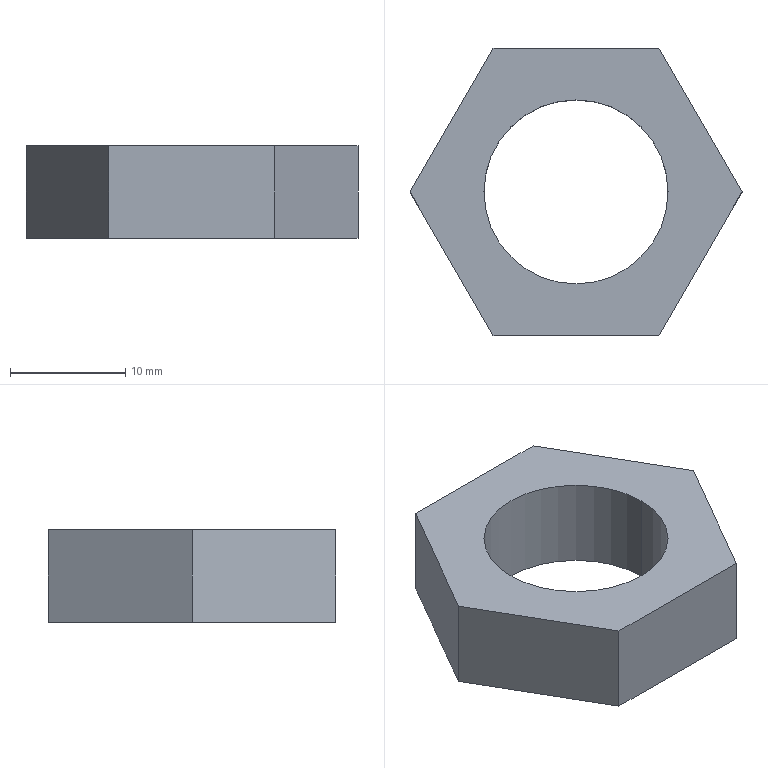Part | STEP file | M16 nut | 1 solid | 10 faces | box 28.868 x 25 x 8 mm | volume 2722 mm3 | plane 8 | cylinder 2 | commonest cylinder face diameters 16 x2
STEP:
#1=CARTESIAN_POINT('',(0.,0.,0.));
#2=DIRECTION('',(0.,0.,1.));
#3=DIRECTION('',(1.,0.,0.));
#4=AXIS2_PLACEMENT_3D('',#1,#2,#3);
#5=CARTESIAN_POINT('',(-8.,0.,8.));
#6=VERTEX_POINT('',#5);
#7=CARTESIAN_POINT('',(-8.,0.,0.));
#8=VERTEX_POINT('',#7);
#9=CARTESIAN_POINT('',(-8.,0.,8.));
#10=DIRECTION('',(0.,0.,-1.));
#11=VECTOR('',#10,1.);
#12=LINE('',#9,#11);
#13=CARTESIAN_POINT('',(0.,0.,8.));
#14=DIRECTION('',(0.,0.,-1.));
#15=DIRECTION('',(-1.,0.,0.));
#16=AXIS2_PLACEMENT_3D('',#13,#14,#15);
#17=CYLINDRICAL_SURFACE('',#16,8.);
#18=CARTESIAN_POINT('',(6.283,0.));
#19=DIRECTION('',(0.,1.));
#20=VECTOR('',#19,1.);
#21=LINE('',#18,#20);
#22=(GEOMETRIC_REPRESENTATION_CONTEXT(2)PARAMETRIC_REPRESENTATION_CONTEXT()REPRESENTATION_CONTEXT('',''));
#23=DEFINITIONAL_REPRESENTATION('',(#21),#22);
#24=PCURVE('',#17,#23);
#25=CARTESIAN_POINT('',(0.,0.,8.));
#26=DIRECTION('',(0.,0.,-1.));
#27=DIRECTION('',(-1.,0.,0.));
#28=AXIS2_PLACEMENT_3D('',#25,#26,#27);
#29=CYLINDRICAL_SURFACE('',#28,8.);
#30=CARTESIAN_POINT('',(0.,0.));
#31=DIRECTION('',(0.,1.));
#32=VECTOR('',#31,1.);
#33=LINE('',#30,#32);
#34=(GEOMETRIC_REPRESENTATION_CONTEXT(2)PARAMETRIC_REPRESENTATION_CONTEXT()REPRESENTATION_CONTEXT('',''));
#35=DEFINITIONAL_REPRESENTATION('',(#33),#34);
#36=PCURVE('',#29,#35);
#37=SURFACE_CURVE('',#12,(#24,#36),.PCURVE_S1.);
#38=EDGE_CURVE('',#6,#8,#37,.T.);
#39=ORIENTED_EDGE('',*,*,#38,.T.);
#40=CARTESIAN_POINT('',(8.,0.,0.));
#41=VERTEX_POINT('',#40);
#42=CARTESIAN_POINT('',(0.,0.,0.));
#43=DIRECTION('',(0.,0.,-1.));
#44=DIRECTION('',(-1.,0.,0.));
#45=AXIS2_PLACEMENT_3D('',#42,#43,#44);
#46=CIRCLE('',#45,8.);
#47=CARTESIAN_POINT('',(0.,8.));
#48=DIRECTION('',(1.,0.));
#49=VECTOR('',#48,1.);
#50=LINE('',#47,#49);
#51=(GEOMETRIC_REPRESENTATION_CONTEXT(2)PARAMETRIC_REPRESENTATION_CONTEXT()REPRESENTATION_CONTEXT('',''));
#52=DEFINITIONAL_REPRESENTATION('',(#50),#51);
#53=PCURVE('',#17,#52);
#54=CARTESIAN_POINT('',(0.,0.,0.));
#55=DIRECTION('',(0.,0.,1.));
#56=DIRECTION('',(1.,0.,0.));
#57=AXIS2_PLACEMENT_3D('',#54,#55,#56);
#58=PLANE('',#57);
#59=CARTESIAN_POINT('',(-8.,0.));
#60=CARTESIAN_POINT('',(-8.,13.856));
#61=CARTESIAN_POINT('',(4.,6.928));
#62=CARTESIAN_POINT('',(16.,0.));
#63=CARTESIAN_POINT('',(4.,-6.928));
#64=CARTESIAN_POINT('',(-8.,-13.856));
#65=CARTESIAN_POINT('',(-8.,0.));
#66=(BOUNDED_CURVE()B_SPLINE_CURVE(2,(#59,#60,#61,#62,#63,#64,#65),.UNSPECIFIED.,.T.,.F.)B_SPLINE_CURVE_WITH_KNOTS((1,2,2,2,2,1),(-2.094,0.,2.094,4.189,6.283,8.378),.UNSPECIFIED.)CURVE()GEOMETRIC_REPRESENTATION_ITEM()RATIONAL_B_SPLINE_CURVE((1.,0.5,1.,0.5,1.,0.5,1.))REPRESENTATION_ITEM(''));
#67=(GEOMETRIC_REPRESENTATION_CONTEXT(2)PARAMETRIC_REPRESENTATION_CONTEXT()REPRESENTATION_CONTEXT('',''));
#68=DEFINITIONAL_REPRESENTATION('',(#66),#67);
#69=PCURVE('',#58,#68);
#70=SURFACE_CURVE('',#46,(#53,#69),.PCURVE_S1.);
#71=EDGE_CURVE('',#41,#8,#70,.T.);
#72=ORIENTED_EDGE('',*,*,#71,.F.);
#73=CARTESIAN_POINT('',(8.,0.,8.));
#74=VERTEX_POINT('',#73);
#75=CARTESIAN_POINT('',(8.,0.,8.));
#76=DIRECTION('',(0.,0.,-1.));
#77=VECTOR('',#76,1.);
#78=LINE('',#75,#77);
#79=CARTESIAN_POINT('',(3.142,0.));
#80=DIRECTION('',(0.,1.));
#81=VECTOR('',#80,1.);
#82=LINE('',#79,#81);
#83=(GEOMETRIC_REPRESENTATION_CONTEXT(2)PARAMETRIC_REPRESENTATION_CONTEXT()REPRESENTATION_CONTEXT('',''));
#84=DEFINITIONAL_REPRESENTATION('',(#82),#83);
#85=PCURVE('',#17,#84);
#86=CARTESIAN_POINT('',(3.142,0.));
#87=DIRECTION('',(0.,1.));
#88=VECTOR('',#87,1.);
#89=LINE('',#86,#88);
#90=(GEOMETRIC_REPRESENTATION_CONTEXT(2)PARAMETRIC_REPRESENTATION_CONTEXT()REPRESENTATION_CONTEXT('',''));
#91=DEFINITIONAL_REPRESENTATION('',(#89),#90);
#92=PCURVE('',#29,#91);
#93=SURFACE_CURVE('',#78,(#85,#92),.PCURVE_S1.);
#94=EDGE_CURVE('',#74,#41,#93,.T.);
#95=ORIENTED_EDGE('',*,*,#94,.F.);
#96=CARTESIAN_POINT('',(0.,0.,8.));
#97=DIRECTION('',(0.,0.,-1.));
#98=DIRECTION('',(-1.,0.,0.));
#99=AXIS2_PLACEMENT_3D('',#96,#97,#98);
#100=CIRCLE('',#99,8.);
#101=CARTESIAN_POINT('',(0.,0.));
#102=DIRECTION('',(1.,0.));
#103=VECTOR('',#102,1.);
#104=LINE('',#101,#103);
#105=(GEOMETRIC_REPRESENTATION_CONTEXT(2)PARAMETRIC_REPRESENTATION_CONTEXT()REPRESENTATION_CONTEXT('',''));
#106=DEFINITIONAL_REPRESENTATION('',(#104),#105);
#107=PCURVE('',#17,#106);
#108=CARTESIAN_POINT('',(0.,0.,8.));
#109=DIRECTION('',(0.,0.,1.));
#110=DIRECTION('',(1.,0.,0.));
#111=AXIS2_PLACEMENT_3D('',#108,#109,#110);
#112=PLANE('',#111);
#113=CARTESIAN_POINT('',(-8.,0.));
#114=CARTESIAN_POINT('',(-8.,13.856));
#115=CARTESIAN_POINT('',(4.,6.928));
#116=CARTESIAN_POINT('',(16.,0.));
#117=CARTESIAN_POINT('',(4.,-6.928));
#118=CARTESIAN_POINT('',(-8.,-13.856));
#119=CARTESIAN_POINT('',(-8.,0.));
#120=(BOUNDED_CURVE()B_SPLINE_CURVE(2,(#113,#114,#115,#116,#117,#118,#119),.UNSPECIFIED.,.T.,.F.)B_SPLINE_CURVE_WITH_KNOTS((1,2,2,2,2,1),(-2.094,0.,2.094,4.189,6.283,8.378),.UNSPECIFIED.)CURVE()GEOMETRIC_REPRESENTATION_ITEM()RATIONAL_B_SPLINE_CURVE((1.,0.5,1.,0.5,1.,0.5,1.))REPRESENTATION_ITEM(''));
#121=(GEOMETRIC_REPRESENTATION_CONTEXT(2)PARAMETRIC_REPRESENTATION_CONTEXT()REPRESENTATION_CONTEXT('',''));
#122=DEFINITIONAL_REPRESENTATION('',(#120),#121);
#123=PCURVE('',#112,#122);
#124=SURFACE_CURVE('',#100,(#107,#123),.PCURVE_S1.);
#125=EDGE_CURVE('',#74,#6,#124,.T.);
#126=ORIENTED_EDGE('',*,*,#125,.T.);
#127=EDGE_LOOP('',(#39,#72,#95,#126));
#128=FACE_BOUND('',#127,.F.);
#129=ADVANCED_FACE('',(#128),#17,.F.);
#130=CARTESIAN_POINT('',(0.,0.,0.));
#131=DIRECTION('',(0.,0.,-1.));
#132=DIRECTION('',(-1.,0.,0.));
#133=AXIS2_PLACEMENT_3D('',#130,#131,#132);
#134=CIRCLE('',#133,8.);
#135=CARTESIAN_POINT('',(-8.,0.));
#136=CARTESIAN_POINT('',(-8.,13.856));
#137=CARTESIAN_POINT('',(4.,6.928));
#138=CARTESIAN_POINT('',(16.,0.));
#139=CARTESIAN_POINT('',(4.,-6.928));
#140=CARTESIAN_POINT('',(-8.,-13.856));
#141=CARTESIAN_POINT('',(-8.,0.));
#142=(BOUNDED_CURVE()B_SPLINE_CURVE(2,(#135,#136,#137,#138,#139,#140,#141),.UNSPECIFIED.,.T.,.F.)B_SPLINE_CURVE_WITH_KNOTS((1,2,2,2,2,1),(-2.094,0.,2.094,4.189,6.283,8.378),.UNSPECIFIED.)CURVE()GEOMETRIC_REPRESENTATION_ITEM()RATIONAL_B_SPLINE_CURVE((1.,0.5,1.,0.5,1.,0.5,1.))REPRESENTATION_ITEM(''));
#143=(GEOMETRIC_REPRESENTATION_CONTEXT(2)PARAMETRIC_REPRESENTATION_CONTEXT()REPRESENTATION_CONTEXT('',''));
#144=DEFINITIONAL_REPRESENTATION('',(#142),#143);
#145=PCURVE('',#58,#144);
#146=CARTESIAN_POINT('',(0.,8.));
#147=DIRECTION('',(1.,0.));
#148=VECTOR('',#147,1.);
#149=LINE('',#146,#148);
#150=(GEOMETRIC_REPRESENTATION_CONTEXT(2)PARAMETRIC_REPRESENTATION_CONTEXT()REPRESENTATION_CONTEXT('',''));
#151=DEFINITIONAL_REPRESENTATION('',(#149),#150);
#152=PCURVE('',#29,#151);
#153=SURFACE_CURVE('',#134,(#145,#152),.PCURVE_S1.);
#154=EDGE_CURVE('',#8,#41,#153,.T.);
#155=ORIENTED_EDGE('',*,*,#154,.F.);
#156=ORIENTED_EDGE('',*,*,#71,.F.);
#157=EDGE_LOOP('',(#155,#156));
#158=FACE_BOUND('',#157,.T.);
#159=CARTESIAN_POINT('',(-7.217,-12.5,0.));
#160=VERTEX_POINT('',#159);
#161=CARTESIAN_POINT('',(7.217,-12.5,0.));
#162=VERTEX_POINT('',#161);
#163=CARTESIAN_POINT('',(0.,-12.5,0.));
#164=DIRECTION('',(1.,0.,0.));
#165=VECTOR('',#164,1.);
#166=LINE('',#163,#165);
#167=CARTESIAN_POINT('',(0.,-12.5));
#168=DIRECTION('',(1.,0.));
#169=VECTOR('',#168,1.);
#170=LINE('',#167,#169);
#171=(GEOMETRIC_REPRESENTATION_CONTEXT(2)PARAMETRIC_REPRESENTATION_CONTEXT()REPRESENTATION_CONTEXT('',''));
#172=DEFINITIONAL_REPRESENTATION('',(#170),#171);
#173=PCURVE('',#58,#172);
#174=CARTESIAN_POINT('',(-7.217,-12.5,8.));
#175=DIRECTION('',(0.,1.,0.));
#176=DIRECTION('',(0.,0.,1.));
#177=AXIS2_PLACEMENT_3D('',#174,#175,#176);
#178=PLANE('',#177);
#179=CARTESIAN_POINT('',(-8.,7.217));
#180=DIRECTION('',(0.,1.));
#181=VECTOR('',#180,1.);
#182=LINE('',#179,#181);
#183=(GEOMETRIC_REPRESENTATION_CONTEXT(2)PARAMETRIC_REPRESENTATION_CONTEXT()REPRESENTATION_CONTEXT('',''));
#184=DEFINITIONAL_REPRESENTATION('',(#182),#183);
#185=PCURVE('',#178,#184);
#186=SURFACE_CURVE('',#166,(#173,#185),.PCURVE_S1.);
#187=EDGE_CURVE('',#160,#162,#186,.T.);
#188=ORIENTED_EDGE('',*,*,#187,.F.);
#189=CARTESIAN_POINT('',(-14.434,0.,0.));
#190=VERTEX_POINT('',#189);
#191=CARTESIAN_POINT('',(-14.434,0.,0.));
#192=DIRECTION('',(0.5,-0.866,0.));
#193=VECTOR('',#192,1.);
#194=LINE('',#191,#193);
#195=CARTESIAN_POINT('',(-14.434,0.));
#196=DIRECTION('',(0.5,-0.866));
#197=VECTOR('',#196,1.);
#198=LINE('',#195,#197);
#199=(GEOMETRIC_REPRESENTATION_CONTEXT(2)PARAMETRIC_REPRESENTATION_CONTEXT()REPRESENTATION_CONTEXT('',''));
#200=DEFINITIONAL_REPRESENTATION('',(#198),#199);
#201=PCURVE('',#58,#200);
#202=CARTESIAN_POINT('',(-14.434,0.,8.));
#203=DIRECTION('',(0.866,0.5,0.));
#204=DIRECTION('',(-0.5,0.866,0.));
#205=AXIS2_PLACEMENT_3D('',#202,#203,#204);
#206=PLANE('',#205);
#207=CARTESIAN_POINT('',(0.,-8.));
#208=DIRECTION('',(-1.,0.));
#209=VECTOR('',#208,1.);
#210=LINE('',#207,#209);
#211=(GEOMETRIC_REPRESENTATION_CONTEXT(2)PARAMETRIC_REPRESENTATION_CONTEXT()REPRESENTATION_CONTEXT('',''));
#212=DEFINITIONAL_REPRESENTATION('',(#210),#211);
#213=PCURVE('',#206,#212);
#214=SURFACE_CURVE('',#194,(#201,#213),.PCURVE_S1.);
#215=EDGE_CURVE('',#190,#160,#214,.T.);
#216=ORIENTED_EDGE('',*,*,#215,.F.);
#217=CARTESIAN_POINT('',(-7.217,12.5,0.));
#218=VERTEX_POINT('',#217);
#219=CARTESIAN_POINT('',(-7.217,12.5,0.));
#220=DIRECTION('',(-0.5,-0.866,0.));
#221=VECTOR('',#220,1.);
#222=LINE('',#219,#221);
#223=CARTESIAN_POINT('',(-7.217,12.5));
#224=DIRECTION('',(-0.5,-0.866));
#225=VECTOR('',#224,1.);
#226=LINE('',#223,#225);
#227=(GEOMETRIC_REPRESENTATION_CONTEXT(2)PARAMETRIC_REPRESENTATION_CONTEXT()REPRESENTATION_CONTEXT('',''));
#228=DEFINITIONAL_REPRESENTATION('',(#226),#227);
#229=PCURVE('',#58,#228);
#230=CARTESIAN_POINT('',(-7.217,12.5,8.));
#231=DIRECTION('',(0.866,-0.5,0.));
#232=DIRECTION('',(0.5,0.866,0.));
#233=AXIS2_PLACEMENT_3D('',#230,#231,#232);
#234=PLANE('',#233);
#235=CARTESIAN_POINT('',(0.,-8.));
#236=DIRECTION('',(-1.,0.));
#237=VECTOR('',#236,1.);
#238=LINE('',#235,#237);
#239=(GEOMETRIC_REPRESENTATION_CONTEXT(2)PARAMETRIC_REPRESENTATION_CONTEXT()REPRESENTATION_CONTEXT('',''));
#240=DEFINITIONAL_REPRESENTATION('',(#238),#239);
#241=PCURVE('',#234,#240);
#242=SURFACE_CURVE('',#222,(#229,#241),.PCURVE_S1.);
#243=EDGE_CURVE('',#218,#190,#242,.T.);
#244=ORIENTED_EDGE('',*,*,#243,.F.);
#245=CARTESIAN_POINT('',(7.217,12.5,0.));
#246=VERTEX_POINT('',#245);
#247=CARTESIAN_POINT('',(0.,12.5,0.));
#248=DIRECTION('',(-1.,0.,0.));
#249=VECTOR('',#248,1.);
#250=LINE('',#247,#249);
#251=CARTESIAN_POINT('',(0.,12.5));
#252=DIRECTION('',(-1.,0.));
#253=VECTOR('',#252,1.);
#254=LINE('',#251,#253);
#255=(GEOMETRIC_REPRESENTATION_CONTEXT(2)PARAMETRIC_REPRESENTATION_CONTEXT()REPRESENTATION_CONTEXT('',''));
#256=DEFINITIONAL_REPRESENTATION('',(#254),#255);
#257=PCURVE('',#58,#256);
#258=CARTESIAN_POINT('',(7.217,12.5,8.));
#259=DIRECTION('',(0.,-1.,0.));
#260=DIRECTION('',(0.,0.,-1.));
#261=AXIS2_PLACEMENT_3D('',#258,#259,#260);
#262=PLANE('',#261);
#263=CARTESIAN_POINT('',(8.,-7.217));
#264=DIRECTION('',(0.,-1.));
#265=VECTOR('',#264,1.);
#266=LINE('',#263,#265);
#267=(GEOMETRIC_REPRESENTATION_CONTEXT(2)PARAMETRIC_REPRESENTATION_CONTEXT()REPRESENTATION_CONTEXT('',''));
#268=DEFINITIONAL_REPRESENTATION('',(#266),#267);
#269=PCURVE('',#262,#268);
#270=SURFACE_CURVE('',#250,(#257,#269),.PCURVE_S1.);
#271=EDGE_CURVE('',#246,#218,#270,.T.);
#272=ORIENTED_EDGE('',*,*,#271,.F.);
#273=CARTESIAN_POINT('',(14.434,0.,0.));
#274=VERTEX_POINT('',#273);
#275=CARTESIAN_POINT('',(14.434,0.,0.));
#276=DIRECTION('',(-0.5,0.866,0.));
#277=VECTOR('',#276,1.);
#278=LINE('',#275,#277);
#279=CARTESIAN_POINT('',(14.434,0.));
#280=DIRECTION('',(-0.5,0.866));
#281=VECTOR('',#280,1.);
#282=LINE('',#279,#281);
#283=(GEOMETRIC_REPRESENTATION_CONTEXT(2)PARAMETRIC_REPRESENTATION_CONTEXT()REPRESENTATION_CONTEXT('',''));
#284=DEFINITIONAL_REPRESENTATION('',(#282),#283);
#285=PCURVE('',#58,#284);
#286=CARTESIAN_POINT('',(14.434,0.,8.));
#287=DIRECTION('',(-0.866,-0.5,0.));
#288=DIRECTION('',(0.5,-0.866,0.));
#289=AXIS2_PLACEMENT_3D('',#286,#287,#288);
#290=PLANE('',#289);
#291=CARTESIAN_POINT('',(0.,-8.));
#292=DIRECTION('',(-1.,0.));
#293=VECTOR('',#292,1.);
#294=LINE('',#291,#293);
#295=(GEOMETRIC_REPRESENTATION_CONTEXT(2)PARAMETRIC_REPRESENTATION_CONTEXT()REPRESENTATION_CONTEXT('',''));
#296=DEFINITIONAL_REPRESENTATION('',(#294),#295);
#297=PCURVE('',#290,#296);
#298=SURFACE_CURVE('',#278,(#285,#297),.PCURVE_S1.);
#299=EDGE_CURVE('',#274,#246,#298,.T.);
#300=ORIENTED_EDGE('',*,*,#299,.F.);
#301=CARTESIAN_POINT('',(7.217,-12.5,0.));
#302=DIRECTION('',(0.5,0.866,0.));
#303=VECTOR('',#302,1.);
#304=LINE('',#301,#303);
#305=CARTESIAN_POINT('',(7.217,-12.5));
#306=DIRECTION('',(0.5,0.866));
#307=VECTOR('',#306,1.);
#308=LINE('',#305,#307);
#309=(GEOMETRIC_REPRESENTATION_CONTEXT(2)PARAMETRIC_REPRESENTATION_CONTEXT()REPRESENTATION_CONTEXT('',''));
#310=DEFINITIONAL_REPRESENTATION('',(#308),#309);
#311=PCURVE('',#58,#310);
#312=CARTESIAN_POINT('',(7.217,-12.5,8.));
#313=DIRECTION('',(-0.866,0.5,0.));
#314=DIRECTION('',(-0.5,-0.866,0.));
#315=AXIS2_PLACEMENT_3D('',#312,#313,#314);
#316=PLANE('',#315);
#317=CARTESIAN_POINT('',(0.,-8.));
#318=DIRECTION('',(-1.,0.));
#319=VECTOR('',#318,1.);
#320=LINE('',#317,#319);
#321=(GEOMETRIC_REPRESENTATION_CONTEXT(2)PARAMETRIC_REPRESENTATION_CONTEXT()REPRESENTATION_CONTEXT('',''));
#322=DEFINITIONAL_REPRESENTATION('',(#320),#321);
#323=PCURVE('',#316,#322);
#324=SURFACE_CURVE('',#304,(#311,#323),.PCURVE_S1.);
#325=EDGE_CURVE('',#162,#274,#324,.T.);
#326=ORIENTED_EDGE('',*,*,#325,.F.);
#327=EDGE_LOOP('',(#188,#216,#244,#272,#300,#326));
#328=FACE_BOUND('',#327,.T.);
#329=ADVANCED_FACE('',(#158,#328),#58,.F.);
#330=ORIENTED_EDGE('',*,*,#154,.F.);
#331=ORIENTED_EDGE('',*,*,#38,.F.);
#332=CARTESIAN_POINT('',(0.,0.,8.));
#333=DIRECTION('',(0.,0.,-1.));
#334=DIRECTION('',(-1.,0.,0.));
#335=AXIS2_PLACEMENT_3D('',#332,#333,#334);
#336=CIRCLE('',#335,8.);
#337=CARTESIAN_POINT('',(0.,0.));
#338=DIRECTION('',(1.,0.));
#339=VECTOR('',#338,1.);
#340=LINE('',#337,#339);
#341=(GEOMETRIC_REPRESENTATION_CONTEXT(2)PARAMETRIC_REPRESENTATION_CONTEXT()REPRESENTATION_CONTEXT('',''));
#342=DEFINITIONAL_REPRESENTATION('',(#340),#341);
#343=PCURVE('',#29,#342);
#344=CARTESIAN_POINT('',(-8.,0.));
#345=CARTESIAN_POINT('',(-8.,13.856));
#346=CARTESIAN_POINT('',(4.,6.928));
#347=CARTESIAN_POINT('',(16.,0.));
#348=CARTESIAN_POINT('',(4.,-6.928));
#349=CARTESIAN_POINT('',(-8.,-13.856));
#350=CARTESIAN_POINT('',(-8.,0.));
#351=(BOUNDED_CURVE()B_SPLINE_CURVE(2,(#344,#345,#346,#347,#348,#349,#350),.UNSPECIFIED.,.T.,.F.)B_SPLINE_CURVE_WITH_KNOTS((1,2,2,2,2,1),(-2.094,0.,2.094,4.189,6.283,8.378),.UNSPECIFIED.)CURVE()GEOMETRIC_REPRESENTATION_ITEM()RATIONAL_B_SPLINE_CURVE((1.,0.5,1.,0.5,1.,0.5,1.))REPRESENTATION_ITEM(''));
#352=(GEOMETRIC_REPRESENTATION_CONTEXT(2)PARAMETRIC_REPRESENTATION_CONTEXT()REPRESENTATION_CONTEXT('',''));
#353=DEFINITIONAL_REPRESENTATION('',(#351),#352);
#354=PCURVE('',#112,#353);
#355=SURFACE_CURVE('',#336,(#343,#354),.PCURVE_S1.);
#356=EDGE_CURVE('',#6,#74,#355,.T.);
#357=ORIENTED_EDGE('',*,*,#356,.T.);
#358=ORIENTED_EDGE('',*,*,#94,.T.);
#359=EDGE_LOOP('',(#330,#331,#357,#358));
#360=FACE_BOUND('',#359,.F.);
#361=ADVANCED_FACE('',(#360),#29,.F.);
#362=CARTESIAN_POINT('',(14.434,0.,8.));
#363=VERTEX_POINT('',#362);
#364=CARTESIAN_POINT('',(14.434,0.,8.));
#365=DIRECTION('',(0.,0.,-1.));
#366=VECTOR('',#365,1.);
#367=LINE('',#364,#366);
#368=CARTESIAN_POINT('',(-14.434,0.));
#369=DIRECTION('',(0.,-1.));
#370=VECTOR('',#369,1.);
#371=LINE('',#368,#370);
#372=(GEOMETRIC_REPRESENTATION_CONTEXT(2)PARAMETRIC_REPRESENTATION_CONTEXT()REPRESENTATION_CONTEXT('',''));
#373=DEFINITIONAL_REPRESENTATION('',(#371),#372);
#374=PCURVE('',#316,#373);
#375=CARTESIAN_POINT('',(0.,0.));
#376=DIRECTION('',(0.,-1.));
#377=VECTOR('',#376,1.);
#378=LINE('',#375,#377);
#379=(GEOMETRIC_REPRESENTATION_CONTEXT(2)PARAMETRIC_REPRESENTATION_CONTEXT()REPRESENTATION_CONTEXT('',''));
#380=DEFINITIONAL_REPRESENTATION('',(#378),#379);
#381=PCURVE('',#290,#380);
#382=SURFACE_CURVE('',#367,(#374,#381),.PCURVE_S1.);
#383=EDGE_CURVE('',#363,#274,#382,.T.);
#384=ORIENTED_EDGE('',*,*,#383,.F.);
#385=CARTESIAN_POINT('',(7.217,-12.5,8.));
#386=VERTEX_POINT('',#385);
#387=CARTESIAN_POINT('',(7.217,-12.5,8.));
#388=DIRECTION('',(0.5,0.866,0.));
#389=VECTOR('',#388,1.);
#390=LINE('',#387,#389);
#391=CARTESIAN_POINT('',(0.,0.));
#392=DIRECTION('',(-1.,0.));
#393=VECTOR('',#392,1.);
#394=LINE('',#391,#393);
#395=(GEOMETRIC_REPRESENTATION_CONTEXT(2)PARAMETRIC_REPRESENTATION_CONTEXT()REPRESENTATION_CONTEXT('',''));
#396=DEFINITIONAL_REPRESENTATION('',(#394),#395);
#397=PCURVE('',#316,#396);
#398=CARTESIAN_POINT('',(7.217,-12.5));
#399=DIRECTION('',(0.5,0.866));
#400=VECTOR('',#399,1.);
#401=LINE('',#398,#400);
#402=(GEOMETRIC_REPRESENTATION_CONTEXT(2)PARAMETRIC_REPRESENTATION_CONTEXT()REPRESENTATION_CONTEXT('',''));
#403=DEFINITIONAL_REPRESENTATION('',(#401),#402);
#404=PCURVE('',#112,#403);
#405=SURFACE_CURVE('',#390,(#397,#404),.PCURVE_S1.);
#406=EDGE_CURVE('',#386,#363,#405,.T.);
#407=ORIENTED_EDGE('',*,*,#406,.F.);
#408=CARTESIAN_POINT('',(7.217,-12.5,8.));
#409=DIRECTION('',(0.,0.,1.));
#410=VECTOR('',#409,1.);
#411=LINE('',#408,#410);
#412=CARTESIAN_POINT('',(0.,0.));
#413=DIRECTION('',(0.,1.));
#414=VECTOR('',#413,1.);
#415=LINE('',#412,#414);
#416=(GEOMETRIC_REPRESENTATION_CONTEXT(2)PARAMETRIC_REPRESENTATION_CONTEXT()REPRESENTATION_CONTEXT('',''));
#417=DEFINITIONAL_REPRESENTATION('',(#415),#416);
#418=PCURVE('',#316,#417);
#419=CARTESIAN_POINT('',(0.,14.434));
#420=DIRECTION('',(1.,0.));
#421=VECTOR('',#420,1.);
#422=LINE('',#419,#421);
#423=(GEOMETRIC_REPRESENTATION_CONTEXT(2)PARAMETRIC_REPRESENTATION_CONTEXT()REPRESENTATION_CONTEXT('',''));
#424=DEFINITIONAL_REPRESENTATION('',(#422),#423);
#425=PCURVE('',#178,#424);
#426=SURFACE_CURVE('',#411,(#418,#425),.PCURVE_S1.);
#427=EDGE_CURVE('',#162,#386,#426,.T.);
#428=ORIENTED_EDGE('',*,*,#427,.F.);
#429=ORIENTED_EDGE('',*,*,#325,.T.);
#430=EDGE_LOOP('',(#384,#407,#428,#429));
#431=FACE_BOUND('',#430,.T.);
#432=ADVANCED_FACE('',(#431),#316,.F.);
#433=ORIENTED_EDGE('',*,*,#427,.T.);
#434=CARTESIAN_POINT('',(-7.217,-12.5,8.));
#435=VERTEX_POINT('',#434);
#436=CARTESIAN_POINT('',(-7.217,-12.5,8.));
#437=DIRECTION('',(1.,0.,0.));
#438=VECTOR('',#437,1.);
#439=LINE('',#436,#438);
#440=CARTESIAN_POINT('',(0.,0.));
#441=DIRECTION('',(0.,1.));
#442=VECTOR('',#441,1.);
#443=LINE('',#440,#442);
#444=(GEOMETRIC_REPRESENTATION_CONTEXT(2)PARAMETRIC_REPRESENTATION_CONTEXT()REPRESENTATION_CONTEXT('',''));
#445=DEFINITIONAL_REPRESENTATION('',(#443),#444);
#446=PCURVE('',#178,#445);
#447=CARTESIAN_POINT('',(-7.217,-12.5));
#448=DIRECTION('',(1.,0.));
#449=VECTOR('',#448,1.);
#450=LINE('',#447,#449);
#451=(GEOMETRIC_REPRESENTATION_CONTEXT(2)PARAMETRIC_REPRESENTATION_CONTEXT()REPRESENTATION_CONTEXT('',''));
#452=DEFINITIONAL_REPRESENTATION('',(#450),#451);
#453=PCURVE('',#112,#452);
#454=SURFACE_CURVE('',#439,(#446,#453),.PCURVE_S1.);
#455=EDGE_CURVE('',#435,#386,#454,.T.);
#456=ORIENTED_EDGE('',*,*,#455,.F.);
#457=CARTESIAN_POINT('',(-7.217,-12.5,8.));
#458=DIRECTION('',(0.,0.,1.));
#459=VECTOR('',#458,1.);
#460=LINE('',#457,#459);
#461=CARTESIAN_POINT('',(0.,0.));
#462=DIRECTION('',(1.,0.));
#463=VECTOR('',#462,1.);
#464=LINE('',#461,#463);
#465=(GEOMETRIC_REPRESENTATION_CONTEXT(2)PARAMETRIC_REPRESENTATION_CONTEXT()REPRESENTATION_CONTEXT('',''));
#466=DEFINITIONAL_REPRESENTATION('',(#464),#465);
#467=PCURVE('',#178,#466);
#468=CARTESIAN_POINT('',(-14.434,0.));
#469=DIRECTION('',(0.,1.));
#470=VECTOR('',#469,1.);
#471=LINE('',#468,#470);
#472=(GEOMETRIC_REPRESENTATION_CONTEXT(2)PARAMETRIC_REPRESENTATION_CONTEXT()REPRESENTATION_CONTEXT('',''));
#473=DEFINITIONAL_REPRESENTATION('',(#471),#472);
#474=PCURVE('',#206,#473);
#475=SURFACE_CURVE('',#460,(#467,#474),.PCURVE_S1.);
#476=EDGE_CURVE('',#160,#435,#475,.T.);
#477=ORIENTED_EDGE('',*,*,#476,.F.);
#478=ORIENTED_EDGE('',*,*,#187,.T.);
#479=EDGE_LOOP('',(#433,#456,#477,#478));
#480=FACE_BOUND('',#479,.T.);
#481=ADVANCED_FACE('',(#480),#178,.F.);
#482=ORIENTED_EDGE('',*,*,#476,.T.);
#483=CARTESIAN_POINT('',(-14.434,0.,8.));
#484=VERTEX_POINT('',#483);
#485=CARTESIAN_POINT('',(-14.434,0.,8.));
#486=DIRECTION('',(0.5,-0.866,0.));
#487=VECTOR('',#486,1.);
#488=LINE('',#485,#487);
#489=CARTESIAN_POINT('',(0.,0.));
#490=DIRECTION('',(-1.,0.));
#491=VECTOR('',#490,1.);
#492=LINE('',#489,#491);
#493=(GEOMETRIC_REPRESENTATION_CONTEXT(2)PARAMETRIC_REPRESENTATION_CONTEXT()REPRESENTATION_CONTEXT('',''));
#494=DEFINITIONAL_REPRESENTATION('',(#492),#493);
#495=PCURVE('',#206,#494);
#496=CARTESIAN_POINT('',(-14.434,0.));
#497=DIRECTION('',(0.5,-0.866));
#498=VECTOR('',#497,1.);
#499=LINE('',#496,#498);
#500=(GEOMETRIC_REPRESENTATION_CONTEXT(2)PARAMETRIC_REPRESENTATION_CONTEXT()REPRESENTATION_CONTEXT('',''));
#501=DEFINITIONAL_REPRESENTATION('',(#499),#500);
#502=PCURVE('',#112,#501);
#503=SURFACE_CURVE('',#488,(#495,#502),.PCURVE_S1.);
#504=EDGE_CURVE('',#484,#435,#503,.T.);
#505=ORIENTED_EDGE('',*,*,#504,.F.);
#506=CARTESIAN_POINT('',(-14.434,0.,8.));
#507=DIRECTION('',(0.,0.,1.));
#508=VECTOR('',#507,1.);
#509=LINE('',#506,#508);
#510=CARTESIAN_POINT('',(0.,0.));
#511=DIRECTION('',(0.,1.));
#512=VECTOR('',#511,1.);
#513=LINE('',#510,#512);
#514=(GEOMETRIC_REPRESENTATION_CONTEXT(2)PARAMETRIC_REPRESENTATION_CONTEXT()REPRESENTATION_CONTEXT('',''));
#515=DEFINITIONAL_REPRESENTATION('',(#513),#514);
#516=PCURVE('',#206,#515);
#517=CARTESIAN_POINT('',(-14.434,0.));
#518=DIRECTION('',(0.,1.));
#519=VECTOR('',#518,1.);
#520=LINE('',#517,#519);
#521=(GEOMETRIC_REPRESENTATION_CONTEXT(2)PARAMETRIC_REPRESENTATION_CONTEXT()REPRESENTATION_CONTEXT('',''));
#522=DEFINITIONAL_REPRESENTATION('',(#520),#521);
#523=PCURVE('',#234,#522);
#524=SURFACE_CURVE('',#509,(#516,#523),.PCURVE_S1.);
#525=EDGE_CURVE('',#190,#484,#524,.T.);
#526=ORIENTED_EDGE('',*,*,#525,.F.);
#527=ORIENTED_EDGE('',*,*,#215,.T.);
#528=EDGE_LOOP('',(#482,#505,#526,#527));
#529=FACE_BOUND('',#528,.T.);
#530=ADVANCED_FACE('',(#529),#206,.F.);
#531=ORIENTED_EDGE('',*,*,#525,.T.);
#532=CARTESIAN_POINT('',(-7.217,12.5,8.));
#533=VERTEX_POINT('',#532);
#534=CARTESIAN_POINT('',(-7.217,12.5,8.));
#535=DIRECTION('',(-0.5,-0.866,0.));
#536=VECTOR('',#535,1.);
#537=LINE('',#534,#536);
#538=CARTESIAN_POINT('',(0.,0.));
#539=DIRECTION('',(-1.,0.));
#540=VECTOR('',#539,1.);
#541=LINE('',#538,#540);
#542=(GEOMETRIC_REPRESENTATION_CONTEXT(2)PARAMETRIC_REPRESENTATION_CONTEXT()REPRESENTATION_CONTEXT('',''));
#543=DEFINITIONAL_REPRESENTATION('',(#541),#542);
#544=PCURVE('',#234,#543);
#545=CARTESIAN_POINT('',(-7.217,12.5));
#546=DIRECTION('',(-0.5,-0.866));
#547=VECTOR('',#546,1.);
#548=LINE('',#545,#547);
#549=(GEOMETRIC_REPRESENTATION_CONTEXT(2)PARAMETRIC_REPRESENTATION_CONTEXT()REPRESENTATION_CONTEXT('',''));
#550=DEFINITIONAL_REPRESENTATION('',(#548),#549);
#551=PCURVE('',#112,#550);
#552=SURFACE_CURVE('',#537,(#544,#551),.PCURVE_S1.);
#553=EDGE_CURVE('',#533,#484,#552,.T.);
#554=ORIENTED_EDGE('',*,*,#553,.F.);
#555=CARTESIAN_POINT('',(-7.217,12.5,8.));
#556=DIRECTION('',(0.,0.,1.));
#557=VECTOR('',#556,1.);
#558=LINE('',#555,#557);
#559=CARTESIAN_POINT('',(0.,0.));
#560=DIRECTION('',(0.,1.));
#561=VECTOR('',#560,1.);
#562=LINE('',#559,#561);
#563=(GEOMETRIC_REPRESENTATION_CONTEXT(2)PARAMETRIC_REPRESENTATION_CONTEXT()REPRESENTATION_CONTEXT('',''));
#564=DEFINITIONAL_REPRESENTATION('',(#562),#563);
#565=PCURVE('',#234,#564);
#566=CARTESIAN_POINT('',(0.,-14.434));
#567=DIRECTION('',(-1.,0.));
#568=VECTOR('',#567,1.);
#569=LINE('',#566,#568);
#570=(GEOMETRIC_REPRESENTATION_CONTEXT(2)PARAMETRIC_REPRESENTATION_CONTEXT()REPRESENTATION_CONTEXT('',''));
#571=DEFINITIONAL_REPRESENTATION('',(#569),#570);
#572=PCURVE('',#262,#571);
#573=SURFACE_CURVE('',#558,(#565,#572),.PCURVE_S1.);
#574=EDGE_CURVE('',#218,#533,#573,.T.);
#575=ORIENTED_EDGE('',*,*,#574,.F.);
#576=ORIENTED_EDGE('',*,*,#243,.T.);
#577=EDGE_LOOP('',(#531,#554,#575,#576));
#578=FACE_BOUND('',#577,.T.);
#579=ADVANCED_FACE('',(#578),#234,.F.);
#580=ORIENTED_EDGE('',*,*,#574,.T.);
#581=CARTESIAN_POINT('',(7.217,12.5,8.));
#582=VERTEX_POINT('',#581);
#583=CARTESIAN_POINT('',(7.217,12.5,8.));
#584=DIRECTION('',(-1.,0.,0.));
#585=VECTOR('',#584,1.);
#586=LINE('',#583,#585);
#587=CARTESIAN_POINT('',(0.,0.));
#588=DIRECTION('',(0.,-1.));
#589=VECTOR('',#588,1.);
#590=LINE('',#587,#589);
#591=(GEOMETRIC_REPRESENTATION_CONTEXT(2)PARAMETRIC_REPRESENTATION_CONTEXT()REPRESENTATION_CONTEXT('',''));
#592=DEFINITIONAL_REPRESENTATION('',(#590),#591);
#593=PCURVE('',#262,#592);
#594=CARTESIAN_POINT('',(7.217,12.5));
#595=DIRECTION('',(-1.,0.));
#596=VECTOR('',#595,1.);
#597=LINE('',#594,#596);
#598=(GEOMETRIC_REPRESENTATION_CONTEXT(2)PARAMETRIC_REPRESENTATION_CONTEXT()REPRESENTATION_CONTEXT('',''));
#599=DEFINITIONAL_REPRESENTATION('',(#597),#598);
#600=PCURVE('',#112,#599);
#601=SURFACE_CURVE('',#586,(#593,#600),.PCURVE_S1.);
#602=EDGE_CURVE('',#582,#533,#601,.T.);
#603=ORIENTED_EDGE('',*,*,#602,.F.);
#604=CARTESIAN_POINT('',(7.217,12.5,8.));
#605=DIRECTION('',(0.,0.,1.));
#606=VECTOR('',#605,1.);
#607=LINE('',#604,#606);
#608=CARTESIAN_POINT('',(0.,0.));
#609=DIRECTION('',(-1.,0.));
#610=VECTOR('',#609,1.);
#611=LINE('',#608,#610);
#612=(GEOMETRIC_REPRESENTATION_CONTEXT(2)PARAMETRIC_REPRESENTATION_CONTEXT()REPRESENTATION_CONTEXT('',''));
#613=DEFINITIONAL_REPRESENTATION('',(#611),#612);
#614=PCURVE('',#262,#613);
#615=CARTESIAN_POINT('',(-14.434,0.));
#616=DIRECTION('',(0.,1.));
#617=VECTOR('',#616,1.);
#618=LINE('',#615,#617);
#619=(GEOMETRIC_REPRESENTATION_CONTEXT(2)PARAMETRIC_REPRESENTATION_CONTEXT()REPRESENTATION_CONTEXT('',''));
#620=DEFINITIONAL_REPRESENTATION('',(#618),#619);
#621=PCURVE('',#290,#620);
#622=SURFACE_CURVE('',#607,(#614,#621),.PCURVE_S1.);
#623=EDGE_CURVE('',#246,#582,#622,.T.);
#624=ORIENTED_EDGE('',*,*,#623,.F.);
#625=ORIENTED_EDGE('',*,*,#271,.T.);
#626=EDGE_LOOP('',(#580,#603,#624,#625));
#627=FACE_BOUND('',#626,.T.);
#628=ADVANCED_FACE('',(#627),#262,.F.);
#629=ORIENTED_EDGE('',*,*,#623,.T.);
#630=CARTESIAN_POINT('',(14.434,0.,8.));
#631=DIRECTION('',(-0.5,0.866,0.));
#632=VECTOR('',#631,1.);
#633=LINE('',#630,#632);
#634=CARTESIAN_POINT('',(0.,0.));
#635=DIRECTION('',(-1.,0.));
#636=VECTOR('',#635,1.);
#637=LINE('',#634,#636);
#638=(GEOMETRIC_REPRESENTATION_CONTEXT(2)PARAMETRIC_REPRESENTATION_CONTEXT()REPRESENTATION_CONTEXT('',''));
#639=DEFINITIONAL_REPRESENTATION('',(#637),#638);
#640=PCURVE('',#290,#639);
#641=CARTESIAN_POINT('',(14.434,0.));
#642=DIRECTION('',(-0.5,0.866));
#643=VECTOR('',#642,1.);
#644=LINE('',#641,#643);
#645=(GEOMETRIC_REPRESENTATION_CONTEXT(2)PARAMETRIC_REPRESENTATION_CONTEXT()REPRESENTATION_CONTEXT('',''));
#646=DEFINITIONAL_REPRESENTATION('',(#644),#645);
#647=PCURVE('',#112,#646);
#648=SURFACE_CURVE('',#633,(#640,#647),.PCURVE_S1.);
#649=EDGE_CURVE('',#363,#582,#648,.T.);
#650=ORIENTED_EDGE('',*,*,#649,.F.);
#651=ORIENTED_EDGE('',*,*,#383,.T.);
#652=ORIENTED_EDGE('',*,*,#299,.T.);
#653=EDGE_LOOP('',(#629,#650,#651,#652));
#654=FACE_BOUND('',#653,.T.);
#655=ADVANCED_FACE('',(#654),#290,.F.);
#656=ORIENTED_EDGE('',*,*,#356,.T.);
#657=ORIENTED_EDGE('',*,*,#125,.T.);
#658=EDGE_LOOP('',(#656,#657));
#659=FACE_BOUND('',#658,.T.);
#660=ORIENTED_EDGE('',*,*,#504,.T.);
#661=ORIENTED_EDGE('',*,*,#455,.T.);
#662=ORIENTED_EDGE('',*,*,#406,.T.);
#663=ORIENTED_EDGE('',*,*,#649,.T.);
#664=ORIENTED_EDGE('',*,*,#602,.T.);
#665=ORIENTED_EDGE('',*,*,#553,.T.);
#666=EDGE_LOOP('',(#660,#661,#662,#663,#664,#665));
#667=FACE_BOUND('',#666,.T.);
#668=ADVANCED_FACE('',(#659,#667),#112,.T.);
#669=CLOSED_SHELL('',(#129,#329,#361,#432,#481,#530,#579,#628,#655,#668));
#670=MANIFOLD_SOLID_BREP('',#669);
#671=(LENGTH_UNIT()NAMED_UNIT(*)SI_UNIT(.MILLI.,.METRE.));
#672=UNCERTAINTY_MEASURE_WITH_UNIT(LENGTH_MEASURE(0.0000001),#671,'','');
#673=(NAMED_UNIT(*)PLANE_ANGLE_UNIT()SI_UNIT($,.RADIAN.));
#674=(NAMED_UNIT(*)SI_UNIT($,.STERADIAN.)SOLID_ANGLE_UNIT());
#675=(GEOMETRIC_REPRESENTATION_CONTEXT(3)GLOBAL_UNCERTAINTY_ASSIGNED_CONTEXT((#672))GLOBAL_UNIT_ASSIGNED_CONTEXT((#671,#673,#674))REPRESENTATION_CONTEXT('',''));
#676=ADVANCED_BREP_SHAPE_REPRESENTATION('',(#4,#670),#675);